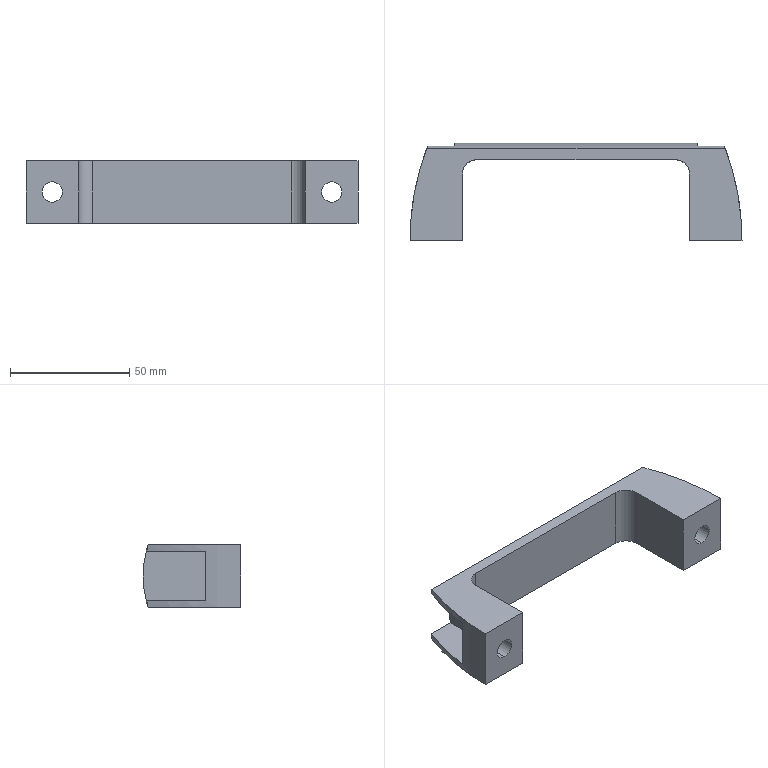Part | STEP file | SecondRearUPCN26-B-41_b_Default | 1 solid | 34 faces | box 139 x 41 x 26 mm | volume 37829 mm3 | cylinder 17 | plane 17 | commonest cylinder face diameters 6 x4 8.5 x4 13.3 x4 12 x2 220.9 x2 82 x1